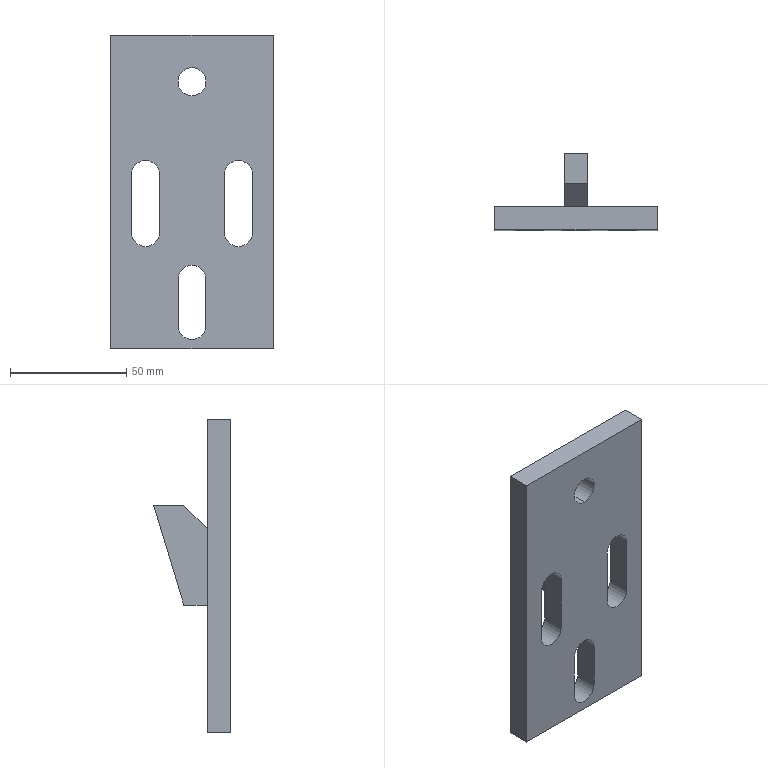Part | SolidWorks | features MirrorStock 1 | 2 solids | 30 faces | box 70 x 33 x 135 mm | volume 88171 mm3 | plane 19 | cylinder 11 | commonest cylinder face diameters 12 x11
STEP:
#1=CARTESIAN_POINT('',(20.,10.,13.5));
#2=VERTEX_POINT('',#1);
#3=CARTESIAN_POINT('',(14.,10.,7.5));
#4=VERTEX_POINT('',#3);
#5=CARTESIAN_POINT('',(20.,10.,7.5));
#6=DIRECTION('',(0.,-1.,0.));
#7=DIRECTION('',(0.,0.,1.));
#8=AXIS2_PLACEMENT_3D('',#5,#6,#7);
#9=CIRCLE('',#8,6.);
#10=EDGE_CURVE('',#2,#4,#9,.T.);
#11=ORIENTED_EDGE('',*,*,#10,.F.);
#12=CARTESIAN_POINT('',(20.,0.,13.5));
#13=VERTEX_POINT('',#12);
#14=CARTESIAN_POINT('',(20.,10.,13.5));
#15=DIRECTION('',(0.,-1.,0.));
#16=VECTOR('',#15,1000.);
#17=LINE('',#14,#16);
#18=EDGE_CURVE('',#2,#13,#17,.T.);
#19=ORIENTED_EDGE('',*,*,#18,.T.);
#20=CARTESIAN_POINT('',(14.,0.,7.5));
#21=VERTEX_POINT('',#20);
#22=CARTESIAN_POINT('',(20.,0.,7.5));
#23=DIRECTION('',(0.,-1.,0.));
#24=DIRECTION('',(0.,0.,1.));
#25=AXIS2_PLACEMENT_3D('',#22,#23,#24);
#26=CIRCLE('',#25,6.);
#27=EDGE_CURVE('',#13,#21,#26,.T.);
#28=ORIENTED_EDGE('',*,*,#27,.T.);
#29=CARTESIAN_POINT('',(14.,10.,7.5));
#30=DIRECTION('',(0.,-1.,0.));
#31=VECTOR('',#30,1000.);
#32=LINE('',#29,#31);
#33=EDGE_CURVE('',#4,#21,#32,.T.);
#34=ORIENTED_EDGE('',*,*,#33,.F.);
#35=EDGE_LOOP('',(#11,#19,#28,#34));
#36=FACE_OUTER_BOUND('',#35,.T.);
#37=CARTESIAN_POINT('',(20.,10.,7.5));
#38=DIRECTION('',(0.,-1.,0.));
#39=DIRECTION('',(0.,0.,1.));
#40=AXIS2_PLACEMENT_3D('',#37,#38,#39);
#41=CYLINDRICAL_SURFACE('',#40,6.);
#42=ADVANCED_FACE('',(#36),#41,.F.);
#43=CARTESIAN_POINT('',(-20.,10.,13.5));
#44=VERTEX_POINT('',#43);
#45=CARTESIAN_POINT('',(-26.,10.,7.5));
#46=VERTEX_POINT('',#45);
#47=CARTESIAN_POINT('',(-20.,10.,7.5));
#48=DIRECTION('',(0.,-1.,0.));
#49=DIRECTION('',(0.,0.,-1.));
#50=AXIS2_PLACEMENT_3D('',#47,#48,#49);
#51=CIRCLE('',#50,6.);
#52=EDGE_CURVE('',#44,#46,#51,.T.);
#53=ORIENTED_EDGE('',*,*,#52,.F.);
#54=CARTESIAN_POINT('',(-20.,0.,13.5));
#55=VERTEX_POINT('',#54);
#56=CARTESIAN_POINT('',(-20.,10.,13.5));
#57=DIRECTION('',(0.,-1.,0.));
#58=VECTOR('',#57,1000.);
#59=LINE('',#56,#58);
#60=EDGE_CURVE('',#44,#55,#59,.T.);
#61=ORIENTED_EDGE('',*,*,#60,.T.);
#62=CARTESIAN_POINT('',(-26.,0.,7.5));
#63=VERTEX_POINT('',#62);
#64=CARTESIAN_POINT('',(-20.,0.,7.5));
#65=DIRECTION('',(0.,-1.,0.));
#66=DIRECTION('',(0.,0.,-1.));
#67=AXIS2_PLACEMENT_3D('',#64,#65,#66);
#68=CIRCLE('',#67,6.);
#69=EDGE_CURVE('',#55,#63,#68,.T.);
#70=ORIENTED_EDGE('',*,*,#69,.T.);
#71=CARTESIAN_POINT('',(-26.,10.,7.5));
#72=DIRECTION('',(0.,-1.,0.));
#73=VECTOR('',#72,1000.);
#74=LINE('',#71,#73);
#75=EDGE_CURVE('',#46,#63,#74,.T.);
#76=ORIENTED_EDGE('',*,*,#75,.F.);
#77=EDGE_LOOP('',(#53,#61,#70,#76));
#78=FACE_OUTER_BOUND('',#77,.T.);
#79=CARTESIAN_POINT('',(-20.,10.,7.5));
#80=DIRECTION('',(0.,-1.,0.));
#81=DIRECTION('',(0.,0.,1.));
#82=AXIS2_PLACEMENT_3D('',#79,#80,#81);
#83=CYLINDRICAL_SURFACE('',#82,6.);
#84=ADVANCED_FACE('',(#78),#83,.F.);
#85=CARTESIAN_POINT('',(0.,10.,-31.5));
#86=VERTEX_POINT('',#85);
#87=CARTESIAN_POINT('',(-6.,10.,-37.5));
#88=VERTEX_POINT('',#87);
#89=CARTESIAN_POINT('',(0.,10.,-37.5));
#90=DIRECTION('',(0.,-1.,0.));
#91=DIRECTION('',(0.,0.,-1.));
#92=AXIS2_PLACEMENT_3D('',#89,#90,#91);
#93=CIRCLE('',#92,6.);
#94=EDGE_CURVE('',#86,#88,#93,.T.);
#95=ORIENTED_EDGE('',*,*,#94,.F.);
#96=CARTESIAN_POINT('',(0.,0.,-31.5));
#97=VERTEX_POINT('',#96);
#98=CARTESIAN_POINT('',(0.,10.,-31.5));
#99=DIRECTION('',(0.,-1.,0.));
#100=VECTOR('',#99,1000.);
#101=LINE('',#98,#100);
#102=EDGE_CURVE('',#86,#97,#101,.T.);
#103=ORIENTED_EDGE('',*,*,#102,.T.);
#104=CARTESIAN_POINT('',(-6.,0.,-37.5));
#105=VERTEX_POINT('',#104);
#106=CARTESIAN_POINT('',(0.,0.,-37.5));
#107=DIRECTION('',(0.,-1.,0.));
#108=DIRECTION('',(0.,0.,-1.));
#109=AXIS2_PLACEMENT_3D('',#106,#107,#108);
#110=CIRCLE('',#109,6.);
#111=EDGE_CURVE('',#97,#105,#110,.T.);
#112=ORIENTED_EDGE('',*,*,#111,.T.);
#113=CARTESIAN_POINT('',(-6.,10.,-37.5));
#114=DIRECTION('',(0.,-1.,0.));
#115=VECTOR('',#114,1000.);
#116=LINE('',#113,#115);
#117=EDGE_CURVE('',#88,#105,#116,.T.);
#118=ORIENTED_EDGE('',*,*,#117,.F.);
#119=EDGE_LOOP('',(#95,#103,#112,#118));
#120=FACE_OUTER_BOUND('',#119,.T.);
#121=CARTESIAN_POINT('',(0.,10.,-37.5));
#122=DIRECTION('',(0.,-1.,0.));
#123=DIRECTION('',(0.,0.,1.));
#124=AXIS2_PLACEMENT_3D('',#121,#122,#123);
#125=CYLINDRICAL_SURFACE('',#124,6.);
#126=ADVANCED_FACE('',(#120),#125,.F.);
#127=CARTESIAN_POINT('',(0.,10.,41.5));
#128=VERTEX_POINT('',#127);
#129=CARTESIAN_POINT('',(0.,10.,53.5));
#130=VERTEX_POINT('',#129);
#131=CARTESIAN_POINT('',(0.,10.,47.5));
#132=DIRECTION('',(0.,-1.,0.));
#133=DIRECTION('',(0.,0.,-1.));
#134=AXIS2_PLACEMENT_3D('',#131,#132,#133);
#135=CIRCLE('',#134,6.);
#136=EDGE_CURVE('',#128,#130,#135,.T.);
#137=ORIENTED_EDGE('',*,*,#136,.F.);
#138=CARTESIAN_POINT('',(0.,0.,41.5));
#139=VERTEX_POINT('',#138);
#140=CARTESIAN_POINT('',(0.,10.,41.5));
#141=DIRECTION('',(0.,-1.,0.));
#142=VECTOR('',#141,1000.);
#143=LINE('',#140,#142);
#144=EDGE_CURVE('',#128,#139,#143,.T.);
#145=ORIENTED_EDGE('',*,*,#144,.T.);
#146=CARTESIAN_POINT('',(0.,0.,53.5));
#147=VERTEX_POINT('',#146);
#148=CARTESIAN_POINT('',(0.,0.,47.5));
#149=DIRECTION('',(0.,-1.,0.));
#150=DIRECTION('',(0.,0.,-1.));
#151=AXIS2_PLACEMENT_3D('',#148,#149,#150);
#152=CIRCLE('',#151,6.);
#153=EDGE_CURVE('',#139,#147,#152,.T.);
#154=ORIENTED_EDGE('',*,*,#153,.T.);
#155=CARTESIAN_POINT('',(0.,10.,53.5));
#156=DIRECTION('',(0.,-1.,0.));
#157=VECTOR('',#156,1000.);
#158=LINE('',#155,#157);
#159=EDGE_CURVE('',#130,#147,#158,.T.);
#160=ORIENTED_EDGE('',*,*,#159,.F.);
#161=EDGE_LOOP('',(#137,#145,#154,#160));
#162=FACE_OUTER_BOUND('',#161,.T.);
#163=CARTESIAN_POINT('',(0.,10.,47.5));
#164=DIRECTION('',(0.,-1.,0.));
#165=DIRECTION('',(0.,0.,1.));
#166=AXIS2_PLACEMENT_3D('',#163,#164,#165);
#167=CYLINDRICAL_SURFACE('',#166,6.);
#168=ADVANCED_FACE('',(#162),#167,.F.);
#169=CARTESIAN_POINT('',(-14.,10.,7.5));
#170=VERTEX_POINT('',#169);
#171=CARTESIAN_POINT('',(-20.,10.,7.5));
#172=DIRECTION('',(0.,-1.,0.));
#173=DIRECTION('',(0.,0.,-1.));
#174=AXIS2_PLACEMENT_3D('',#171,#172,#173);
#175=CIRCLE('',#174,6.);
#176=EDGE_CURVE('',#170,#44,#175,.T.);
#177=ORIENTED_EDGE('',*,*,#176,.T.);
#178=ORIENTED_EDGE('',*,*,#52,.T.);
#179=CARTESIAN_POINT('',(-26.,10.,-17.5));
#180=VERTEX_POINT('',#179);
#181=CARTESIAN_POINT('',(-26.,10.,7.5));
#182=DIRECTION('',(0.,0.,-1.));
#183=VECTOR('',#182,1000.);
#184=LINE('',#181,#183);
#185=EDGE_CURVE('',#46,#180,#184,.T.);
#186=ORIENTED_EDGE('',*,*,#185,.T.);
#187=CARTESIAN_POINT('',(-14.,10.,-17.5));
#188=VERTEX_POINT('',#187);
#189=CARTESIAN_POINT('',(-20.,10.,-17.5));
#190=DIRECTION('',(0.,-1.,0.));
#191=DIRECTION('',(0.,0.,-1.));
#192=AXIS2_PLACEMENT_3D('',#189,#190,#191);
#193=CIRCLE('',#192,6.);
#194=EDGE_CURVE('',#180,#188,#193,.T.);
#195=ORIENTED_EDGE('',*,*,#194,.T.);
#196=CARTESIAN_POINT('',(-14.,10.,7.5));
#197=DIRECTION('',(0.,0.,1.));
#198=VECTOR('',#197,1000.);
#199=LINE('',#196,#198);
#200=EDGE_CURVE('',#188,#170,#199,.T.);
#201=ORIENTED_EDGE('',*,*,#200,.T.);
#202=EDGE_LOOP('',(#177,#178,#186,#195,#201));
#203=FACE_BOUND('',#202,.T.);
#204=CARTESIAN_POINT('',(0.,10.,47.5));
#205=DIRECTION('',(0.,-1.,0.));
#206=DIRECTION('',(0.,0.,-1.));
#207=AXIS2_PLACEMENT_3D('',#204,#205,#206);
#208=CIRCLE('',#207,6.);
#209=EDGE_CURVE('',#130,#128,#208,.T.);
#210=ORIENTED_EDGE('',*,*,#209,.T.);
#211=ORIENTED_EDGE('',*,*,#136,.T.);
#212=EDGE_LOOP('',(#210,#211));
#213=FACE_BOUND('',#212,.T.);
#214=CARTESIAN_POINT('',(35.,10.,-67.5));
#215=VERTEX_POINT('',#214);
#216=CARTESIAN_POINT('',(35.,10.,67.5));
#217=VERTEX_POINT('',#216);
#218=CARTESIAN_POINT('',(35.,10.,-67.5));
#219=DIRECTION('',(0.,0.,1.));
#220=VECTOR('',#219,1000.);
#221=LINE('',#218,#220);
#222=EDGE_CURVE('',#215,#217,#221,.T.);
#223=ORIENTED_EDGE('',*,*,#222,.F.);
#224=CARTESIAN_POINT('',(-35.,10.,-67.5));
#225=VERTEX_POINT('',#224);
#226=CARTESIAN_POINT('',(-35.,10.,-67.5));
#227=DIRECTION('',(1.,0.,0.));
#228=VECTOR('',#227,1000.);
#229=LINE('',#226,#228);
#230=EDGE_CURVE('',#225,#215,#229,.T.);
#231=ORIENTED_EDGE('',*,*,#230,.F.);
#232=CARTESIAN_POINT('',(-35.,10.,67.5));
#233=VERTEX_POINT('',#232);
#234=CARTESIAN_POINT('',(-35.,10.,-67.5));
#235=DIRECTION('',(0.,0.,-1.));
#236=VECTOR('',#235,1000.);
#237=LINE('',#234,#236);
#238=EDGE_CURVE('',#233,#225,#237,.T.);
#239=ORIENTED_EDGE('',*,*,#238,.F.);
#240=CARTESIAN_POINT('',(-35.,10.,67.5));
#241=DIRECTION('',(-1.,0.,0.));
#242=VECTOR('',#241,1000.);
#243=LINE('',#240,#242);
#244=EDGE_CURVE('',#217,#233,#243,.T.);
#245=ORIENTED_EDGE('',*,*,#244,.F.);
#246=EDGE_LOOP('',(#223,#231,#239,#245));
#247=FACE_OUTER_BOUND('',#246,.T.);
#248=CARTESIAN_POINT('',(6.,10.,-37.5));
#249=VERTEX_POINT('',#248);
#250=CARTESIAN_POINT('',(0.,10.,-37.5));
#251=DIRECTION('',(0.,-1.,0.));
#252=DIRECTION('',(0.,0.,-1.));
#253=AXIS2_PLACEMENT_3D('',#250,#251,#252);
#254=CIRCLE('',#253,6.);
#255=EDGE_CURVE('',#249,#86,#254,.T.);
#256=ORIENTED_EDGE('',*,*,#255,.T.);
#257=ORIENTED_EDGE('',*,*,#94,.T.);
#258=CARTESIAN_POINT('',(-6.,10.,-57.5));
#259=VERTEX_POINT('',#258);
#260=CARTESIAN_POINT('',(-6.,10.,-37.5));
#261=DIRECTION('',(0.,0.,-1.));
#262=VECTOR('',#261,1000.);
#263=LINE('',#260,#262);
#264=EDGE_CURVE('',#88,#259,#263,.T.);
#265=ORIENTED_EDGE('',*,*,#264,.T.);
#266=CARTESIAN_POINT('',(6.,10.,-57.5));
#267=VERTEX_POINT('',#266);
#268=CARTESIAN_POINT('',(0.,10.,-57.5));
#269=DIRECTION('',(0.,-1.,0.));
#270=DIRECTION('',(0.,0.,-1.));
#271=AXIS2_PLACEMENT_3D('',#268,#269,#270);
#272=CIRCLE('',#271,6.);
#273=EDGE_CURVE('',#259,#267,#272,.T.);
#274=ORIENTED_EDGE('',*,*,#273,.T.);
#275=CARTESIAN_POINT('',(6.,10.,-37.5));
#276=DIRECTION('',(0.,0.,1.));
#277=VECTOR('',#276,1000.);
#278=LINE('',#275,#277);
#279=EDGE_CURVE('',#267,#249,#278,.T.);
#280=ORIENTED_EDGE('',*,*,#279,.T.);
#281=EDGE_LOOP('',(#256,#257,#265,#274,#280));
#282=FACE_BOUND('',#281,.T.);
#283=CARTESIAN_POINT('',(26.,10.,7.5));
#284=VERTEX_POINT('',#283);
#285=CARTESIAN_POINT('',(20.,10.,7.5));
#286=DIRECTION('',(0.,-1.,0.));
#287=DIRECTION('',(0.,0.,1.));
#288=AXIS2_PLACEMENT_3D('',#285,#286,#287);
#289=CIRCLE('',#288,6.);
#290=EDGE_CURVE('',#284,#2,#289,.T.);
#291=ORIENTED_EDGE('',*,*,#290,.T.);
#292=ORIENTED_EDGE('',*,*,#10,.T.);
#293=CARTESIAN_POINT('',(14.,10.,-17.5));
#294=VERTEX_POINT('',#293);
#295=CARTESIAN_POINT('',(14.,10.,7.5));
#296=DIRECTION('',(0.,0.,-1.));
#297=VECTOR('',#296,1000.);
#298=LINE('',#295,#297);
#299=EDGE_CURVE('',#4,#294,#298,.T.);
#300=ORIENTED_EDGE('',*,*,#299,.T.);
#301=CARTESIAN_POINT('',(26.,10.,-17.5));
#302=VERTEX_POINT('',#301);
#303=CARTESIAN_POINT('',(20.,10.,-17.5));
#304=DIRECTION('',(0.,-1.,0.));
#305=DIRECTION('',(0.,0.,1.));
#306=AXIS2_PLACEMENT_3D('',#303,#304,#305);
#307=CIRCLE('',#306,6.);
#308=EDGE_CURVE('',#294,#302,#307,.T.);
#309=ORIENTED_EDGE('',*,*,#308,.T.);
#310=CARTESIAN_POINT('',(26.,10.,7.5));
#311=DIRECTION('',(0.,0.,1.));
#312=VECTOR('',#311,1000.);
#313=LINE('',#310,#312);
#314=EDGE_CURVE('',#302,#284,#313,.T.);
#315=ORIENTED_EDGE('',*,*,#314,.T.);
#316=EDGE_LOOP('',(#291,#292,#300,#309,#315));
#317=FACE_BOUND('',#316,.T.);
#318=CARTESIAN_POINT('',(0.,10.,0.));
#319=DIRECTION('',(0.,-1.,0.));
#320=DIRECTION('',(0.,0.,1.));
#321=AXIS2_PLACEMENT_3D('',#318,#319,#320);
#322=PLANE('',#321);
#323=ADVANCED_FACE('',(#203,#213,#247,#282,#317),#322,.F.);
#324=CARTESIAN_POINT('',(35.,0.,-67.5));
#325=VERTEX_POINT('',#324);
#326=CARTESIAN_POINT('',(35.,0.,67.5));
#327=VERTEX_POINT('',#326);
#328=CARTESIAN_POINT('',(35.,0.,-67.5));
#329=DIRECTION('',(0.,0.,1.));
#330=VECTOR('',#329,1000.);
#331=LINE('',#328,#330);
#332=EDGE_CURVE('',#325,#327,#331,.T.);
#333=ORIENTED_EDGE('',*,*,#332,.T.);
#334=CARTESIAN_POINT('',(-35.,0.,67.5));
#335=VERTEX_POINT('',#334);
#336=CARTESIAN_POINT('',(-35.,0.,67.5));
#337=DIRECTION('',(-1.,0.,0.));
#338=VECTOR('',#337,1000.);
#339=LINE('',#336,#338);
#340=EDGE_CURVE('',#327,#335,#339,.T.);
#341=ORIENTED_EDGE('',*,*,#340,.T.);
#342=CARTESIAN_POINT('',(-35.,0.,-67.5));
#343=VERTEX_POINT('',#342);
#344=CARTESIAN_POINT('',(-35.,0.,-67.5));
#345=DIRECTION('',(0.,0.,-1.));
#346=VECTOR('',#345,1000.);
#347=LINE('',#344,#346);
#348=EDGE_CURVE('',#335,#343,#347,.T.);
#349=ORIENTED_EDGE('',*,*,#348,.T.);
#350=CARTESIAN_POINT('',(-35.,0.,-67.5));
#351=DIRECTION('',(1.,0.,0.));
#352=VECTOR('',#351,1000.);
#353=LINE('',#350,#352);
#354=EDGE_CURVE('',#343,#325,#353,.T.);
#355=ORIENTED_EDGE('',*,*,#354,.T.);
#356=EDGE_LOOP('',(#333,#341,#349,#355));
#357=FACE_OUTER_BOUND('',#356,.T.);
#358=CARTESIAN_POINT('',(0.,0.,47.5));
#359=DIRECTION('',(0.,-1.,0.));
#360=DIRECTION('',(0.,0.,-1.));
#361=AXIS2_PLACEMENT_3D('',#358,#359,#360);
#362=CIRCLE('',#361,6.);
#363=EDGE_CURVE('',#147,#139,#362,.T.);
#364=ORIENTED_EDGE('',*,*,#363,.F.);
#365=ORIENTED_EDGE('',*,*,#153,.F.);
#366=EDGE_LOOP('',(#364,#365));
#367=FACE_BOUND('',#366,.T.);
#368=CARTESIAN_POINT('',(6.,0.,-57.5));
#369=VERTEX_POINT('',#368);
#370=CARTESIAN_POINT('',(6.,0.,-37.5));
#371=VERTEX_POINT('',#370);
#372=CARTESIAN_POINT('',(6.,0.,-37.5));
#373=DIRECTION('',(0.,0.,1.));
#374=VECTOR('',#373,1000.);
#375=LINE('',#372,#374);
#376=EDGE_CURVE('',#369,#371,#375,.T.);
#377=ORIENTED_EDGE('',*,*,#376,.F.);
#378=CARTESIAN_POINT('',(-6.,0.,-57.5));
#379=VERTEX_POINT('',#378);
#380=CARTESIAN_POINT('',(0.,0.,-57.5));
#381=DIRECTION('',(0.,-1.,0.));
#382=DIRECTION('',(0.,0.,-1.));
#383=AXIS2_PLACEMENT_3D('',#380,#381,#382);
#384=CIRCLE('',#383,6.);
#385=EDGE_CURVE('',#379,#369,#384,.T.);
#386=ORIENTED_EDGE('',*,*,#385,.F.);
#387=CARTESIAN_POINT('',(-6.,0.,-37.5));
#388=DIRECTION('',(0.,0.,-1.));
#389=VECTOR('',#388,1000.);
#390=LINE('',#387,#389);
#391=EDGE_CURVE('',#105,#379,#390,.T.);
#392=ORIENTED_EDGE('',*,*,#391,.F.);
#393=ORIENTED_EDGE('',*,*,#111,.F.);
#394=CARTESIAN_POINT('',(0.,0.,-37.5));
#395=DIRECTION('',(0.,-1.,0.));
#396=DIRECTION('',(0.,0.,-1.));
#397=AXIS2_PLACEMENT_3D('',#394,#395,#396);
#398=CIRCLE('',#397,6.);
#399=EDGE_CURVE('',#371,#97,#398,.T.);
#400=ORIENTED_EDGE('',*,*,#399,.F.);
#401=EDGE_LOOP('',(#377,#386,#392,#393,#400));
#402=FACE_BOUND('',#401,.T.);
#403=CARTESIAN_POINT('',(-14.,0.,-17.5));
#404=VERTEX_POINT('',#403);
#405=CARTESIAN_POINT('',(-14.,0.,7.5));
#406=VERTEX_POINT('',#405);
#407=CARTESIAN_POINT('',(-14.,0.,7.5));
#408=DIRECTION('',(0.,0.,1.));
#409=VECTOR('',#408,1000.);
#410=LINE('',#407,#409);
#411=EDGE_CURVE('',#404,#406,#410,.T.);
#412=ORIENTED_EDGE('',*,*,#411,.F.);
#413=CARTESIAN_POINT('',(-26.,0.,-17.5));
#414=VERTEX_POINT('',#413);
#415=CARTESIAN_POINT('',(-20.,0.,-17.5));
#416=DIRECTION('',(0.,-1.,0.));
#417=DIRECTION('',(0.,0.,-1.));
#418=AXIS2_PLACEMENT_3D('',#415,#416,#417);
#419=CIRCLE('',#418,6.);
#420=EDGE_CURVE('',#414,#404,#419,.T.);
#421=ORIENTED_EDGE('',*,*,#420,.F.);
#422=CARTESIAN_POINT('',(-26.,0.,7.5));
#423=DIRECTION('',(0.,0.,-1.));
#424=VECTOR('',#423,1000.);
#425=LINE('',#422,#424);
#426=EDGE_CURVE('',#63,#414,#425,.T.);
#427=ORIENTED_EDGE('',*,*,#426,.F.);
#428=ORIENTED_EDGE('',*,*,#69,.F.);
#429=CARTESIAN_POINT('',(-20.,0.,7.5));
#430=DIRECTION('',(0.,-1.,0.));
#431=DIRECTION('',(0.,0.,-1.));
#432=AXIS2_PLACEMENT_3D('',#429,#430,#431);
#433=CIRCLE('',#432,6.);
#434=EDGE_CURVE('',#406,#55,#433,.T.);
#435=ORIENTED_EDGE('',*,*,#434,.F.);
#436=EDGE_LOOP('',(#412,#421,#427,#428,#435));
#437=FACE_BOUND('',#436,.T.);
#438=CARTESIAN_POINT('',(26.,0.,-17.5));
#439=VERTEX_POINT('',#438);
#440=CARTESIAN_POINT('',(26.,0.,7.5));
#441=VERTEX_POINT('',#440);
#442=CARTESIAN_POINT('',(26.,0.,7.5));
#443=DIRECTION('',(0.,0.,1.));
#444=VECTOR('',#443,1000.);
#445=LINE('',#442,#444);
#446=EDGE_CURVE('',#439,#441,#445,.T.);
#447=ORIENTED_EDGE('',*,*,#446,.F.);
#448=CARTESIAN_POINT('',(14.,0.,-17.5));
#449=VERTEX_POINT('',#448);
#450=CARTESIAN_POINT('',(20.,0.,-17.5));
#451=DIRECTION('',(0.,-1.,0.));
#452=DIRECTION('',(0.,0.,1.));
#453=AXIS2_PLACEMENT_3D('',#450,#451,#452);
#454=CIRCLE('',#453,6.);
#455=EDGE_CURVE('',#449,#439,#454,.T.);
#456=ORIENTED_EDGE('',*,*,#455,.F.);
#457=CARTESIAN_POINT('',(14.,0.,7.5));
#458=DIRECTION('',(0.,0.,-1.));
#459=VECTOR('',#458,1000.);
#460=LINE('',#457,#459);
#461=EDGE_CURVE('',#21,#449,#460,.T.);
#462=ORIENTED_EDGE('',*,*,#461,.F.);
#463=ORIENTED_EDGE('',*,*,#27,.F.);
#464=CARTESIAN_POINT('',(20.,0.,7.5));
#465=DIRECTION('',(0.,-1.,0.));
#466=DIRECTION('',(0.,0.,1.));
#467=AXIS2_PLACEMENT_3D('',#464,#465,#466);
#468=CIRCLE('',#467,6.);
#469=EDGE_CURVE('',#441,#13,#468,.T.);
#470=ORIENTED_EDGE('',*,*,#469,.F.);
#471=EDGE_LOOP('',(#447,#456,#462,#463,#470));
#472=FACE_BOUND('',#471,.T.);
#473=CARTESIAN_POINT('',(0.,0.,0.));
#474=DIRECTION('',(0.,-1.,0.));
#475=DIRECTION('',(0.,0.,1.));
#476=AXIS2_PLACEMENT_3D('',#473,#474,#475);
#477=PLANE('',#476);
#478=ADVANCED_FACE('',(#357,#367,#402,#437,#472),#477,.T.);
#479=ORIENTED_EDGE('',*,*,#332,.F.);
#480=CARTESIAN_POINT('',(35.,10.,-67.5));
#481=DIRECTION('',(0.,-1.,0.));
#482=VECTOR('',#481,1000.);
#483=LINE('',#480,#482);
#484=EDGE_CURVE('',#215,#325,#483,.T.);
#485=ORIENTED_EDGE('',*,*,#484,.F.);
#486=ORIENTED_EDGE('',*,*,#222,.T.);
#487=CARTESIAN_POINT('',(35.,10.,67.5));
#488=DIRECTION('',(0.,-1.,0.));
#489=VECTOR('',#488,1000.);
#490=LINE('',#487,#489);
#491=EDGE_CURVE('',#217,#327,#490,.T.);
#492=ORIENTED_EDGE('',*,*,#491,.T.);
#493=EDGE_LOOP('',(#479,#485,#486,#492));
#494=FACE_OUTER_BOUND('',#493,.T.);
#495=CARTESIAN_POINT('',(35.,10.,-67.5));
#496=DIRECTION('',(-1.,0.,0.));
#497=DIRECTION('',(0.,0.,-1.));
#498=AXIS2_PLACEMENT_3D('',#495,#496,#497);
#499=PLANE('',#498);
#500=ADVANCED_FACE('',(#494),#499,.F.);
#501=ORIENTED_EDGE('',*,*,#340,.F.);
#502=ORIENTED_EDGE('',*,*,#491,.F.);
#503=ORIENTED_EDGE('',*,*,#244,.T.);
#504=CARTESIAN_POINT('',(-35.,10.,67.5));
#505=DIRECTION('',(0.,-1.,0.));
#506=VECTOR('',#505,1000.);
#507=LINE('',#504,#506);
#508=EDGE_CURVE('',#233,#335,#507,.T.);
#509=ORIENTED_EDGE('',*,*,#508,.T.);
#510=EDGE_LOOP('',(#501,#502,#503,#509));
#511=FACE_OUTER_BOUND('',#510,.T.);
#512=CARTESIAN_POINT('',(-35.,10.,67.5));
#513=DIRECTION('',(0.,0.,-1.));
#514=DIRECTION('',(1.,0.,0.));
#515=AXIS2_PLACEMENT_3D('',#512,#513,#514);
#516=PLANE('',#515);
#517=ADVANCED_FACE('',(#511),#516,.F.);
#518=ORIENTED_EDGE('',*,*,#348,.F.);
#519=ORIENTED_EDGE('',*,*,#508,.F.);
#520=ORIENTED_EDGE('',*,*,#238,.T.);
#521=CARTESIAN_POINT('',(-35.,10.,-67.5));
#522=DIRECTION('',(0.,-1.,0.));
#523=VECTOR('',#522,1000.);
#524=LINE('',#521,#523);
#525=EDGE_CURVE('',#225,#343,#524,.T.);
#526=ORIENTED_EDGE('',*,*,#525,.T.);
#527=EDGE_LOOP('',(#518,#519,#520,#526));
#528=FACE_OUTER_BOUND('',#527,.T.);
#529=CARTESIAN_POINT('',(-35.,10.,-67.5));
#530=DIRECTION('',(1.,0.,0.));
#531=DIRECTION('',(0.,0.,1.));
#532=AXIS2_PLACEMENT_3D('',#529,#530,#531);
#533=PLANE('',#532);
#534=ADVANCED_FACE('',(#528),#533,.F.);
#535=ORIENTED_EDGE('',*,*,#354,.F.);
#536=ORIENTED_EDGE('',*,*,#525,.F.);
#537=ORIENTED_EDGE('',*,*,#230,.T.);
#538=ORIENTED_EDGE('',*,*,#484,.T.);
#539=EDGE_LOOP('',(#535,#536,#537,#538));
#540=FACE_OUTER_BOUND('',#539,.T.);
#541=CARTESIAN_POINT('',(-35.,10.,-67.5));
#542=DIRECTION('',(0.,0.,1.));
#543=DIRECTION('',(-1.,0.,0.));
#544=AXIS2_PLACEMENT_3D('',#541,#542,#543);
#545=PLANE('',#544);
#546=ADVANCED_FACE('',(#540),#545,.F.);
#547=ORIENTED_EDGE('',*,*,#144,.F.);
#548=ORIENTED_EDGE('',*,*,#209,.F.);
#549=ORIENTED_EDGE('',*,*,#159,.T.);
#550=ORIENTED_EDGE('',*,*,#363,.T.);
#551=EDGE_LOOP('',(#547,#548,#549,#550));
#552=FACE_OUTER_BOUND('',#551,.T.);
#553=CARTESIAN_POINT('',(0.,10.,47.5));
#554=DIRECTION('',(0.,-1.,0.));
#555=DIRECTION('',(0.,0.,1.));
#556=AXIS2_PLACEMENT_3D('',#553,#554,#555);
#557=CYLINDRICAL_SURFACE('',#556,6.);
#558=ADVANCED_FACE('',(#552),#557,.F.);
#559=ORIENTED_EDGE('',*,*,#102,.F.);
#560=ORIENTED_EDGE('',*,*,#255,.F.);
#561=CARTESIAN_POINT('',(6.,10.,-37.5));
#562=DIRECTION('',(0.,-1.,0.));
#563=VECTOR('',#562,1000.);
#564=LINE('',#561,#563);
#565=EDGE_CURVE('',#249,#371,#564,.T.);
#566=ORIENTED_EDGE('',*,*,#565,.T.);
#567=ORIENTED_EDGE('',*,*,#399,.T.);
#568=EDGE_LOOP('',(#559,#560,#566,#567));
#569=FACE_OUTER_BOUND('',#568,.T.);
#570=CARTESIAN_POINT('',(0.,10.,-37.5));
#571=DIRECTION('',(0.,-1.,0.));
#572=DIRECTION('',(0.,0.,1.));
#573=AXIS2_PLACEMENT_3D('',#570,#571,#572);
#574=CYLINDRICAL_SURFACE('',#573,6.);
#575=ADVANCED_FACE('',(#569),#574,.F.);
#576=ORIENTED_EDGE('',*,*,#391,.T.);
#577=CARTESIAN_POINT('',(-6.,10.,-57.5));
#578=DIRECTION('',(0.,-1.,0.));
#579=VECTOR('',#578,1000.);
#580=LINE('',#577,#579);
#581=EDGE_CURVE('',#259,#379,#580,.T.);
#582=ORIENTED_EDGE('',*,*,#581,.F.);
#583=ORIENTED_EDGE('',*,*,#264,.F.);
#584=ORIENTED_EDGE('',*,*,#117,.T.);
#585=EDGE_LOOP('',(#576,#582,#583,#584));
#586=FACE_OUTER_BOUND('',#585,.T.);
#587=CARTESIAN_POINT('',(-6.,10.,-37.5));
#588=DIRECTION('',(1.,0.,0.));
#589=DIRECTION('',(0.,0.,1.));
#590=AXIS2_PLACEMENT_3D('',#587,#588,#589);
#591=PLANE('',#590);
#592=ADVANCED_FACE('',(#586),#591,.T.);
#593=ORIENTED_EDGE('',*,*,#385,.T.);
#594=CARTESIAN_POINT('',(6.,10.,-57.5));
#595=DIRECTION('',(0.,-1.,0.));
#596=VECTOR('',#595,1000.);
#597=LINE('',#594,#596);
#598=EDGE_CURVE('',#267,#369,#597,.T.);
#599=ORIENTED_EDGE('',*,*,#598,.F.);
#600=ORIENTED_EDGE('',*,*,#273,.F.);
#601=ORIENTED_EDGE('',*,*,#581,.T.);
#602=EDGE_LOOP('',(#593,#599,#600,#601));
#603=FACE_OUTER_BOUND('',#602,.T.);
#604=CARTESIAN_POINT('',(0.,10.,-57.5));
#605=DIRECTION('',(0.,-1.,0.));
#606=DIRECTION('',(0.,0.,1.));
#607=AXIS2_PLACEMENT_3D('',#604,#605,#606);
#608=CYLINDRICAL_SURFACE('',#607,6.);
#609=ADVANCED_FACE('',(#603),#608,.F.);
#610=ORIENTED_EDGE('',*,*,#376,.T.);
#611=ORIENTED_EDGE('',*,*,#565,.F.);
#612=ORIENTED_EDGE('',*,*,#279,.F.);
#613=ORIENTED_EDGE('',*,*,#598,.T.);
#614=EDGE_LOOP('',(#610,#611,#612,#613));
#615=FACE_OUTER_BOUND('',#614,.T.);
#616=CARTESIAN_POINT('',(6.,10.,-37.5));
#617=DIRECTION('',(-1.,0.,0.));
#618=DIRECTION('',(0.,0.,-1.));
#619=AXIS2_PLACEMENT_3D('',#616,#617,#618);
#620=PLANE('',#619);
#621=ADVANCED_FACE('',(#615),#620,.T.);
#622=ORIENTED_EDGE('',*,*,#60,.F.);
#623=ORIENTED_EDGE('',*,*,#176,.F.);
#624=CARTESIAN_POINT('',(-14.,10.,7.5));
#625=DIRECTION('',(0.,-1.,0.));
#626=VECTOR('',#625,1000.);
#627=LINE('',#624,#626);
#628=EDGE_CURVE('',#170,#406,#627,.T.);
#629=ORIENTED_EDGE('',*,*,#628,.T.);
#630=ORIENTED_EDGE('',*,*,#434,.T.);
#631=EDGE_LOOP('',(#622,#623,#629,#630));
#632=FACE_OUTER_BOUND('',#631,.T.);
#633=CARTESIAN_POINT('',(-20.,10.,7.5));
#634=DIRECTION('',(0.,-1.,0.));
#635=DIRECTION('',(0.,0.,1.));
#636=AXIS2_PLACEMENT_3D('',#633,#634,#635);
#637=CYLINDRICAL_SURFACE('',#636,6.);
#638=ADVANCED_FACE('',(#632),#637,.F.);
#639=ORIENTED_EDGE('',*,*,#426,.T.);
#640=CARTESIAN_POINT('',(-26.,10.,-17.5));
#641=DIRECTION('',(0.,-1.,0.));
#642=VECTOR('',#641,1000.);
#643=LINE('',#640,#642);
#644=EDGE_CURVE('',#180,#414,#643,.T.);
#645=ORIENTED_EDGE('',*,*,#644,.F.);
#646=ORIENTED_EDGE('',*,*,#185,.F.);
#647=ORIENTED_EDGE('',*,*,#75,.T.);
#648=EDGE_LOOP('',(#639,#645,#646,#647));
#649=FACE_OUTER_BOUND('',#648,.T.);
#650=CARTESIAN_POINT('',(-26.,10.,7.5));
#651=DIRECTION('',(1.,0.,0.));
#652=DIRECTION('',(0.,0.,1.));
#653=AXIS2_PLACEMENT_3D('',#650,#651,#652);
#654=PLANE('',#653);
#655=ADVANCED_FACE('',(#649),#654,.T.);
#656=ORIENTED_EDGE('',*,*,#420,.T.);
#657=CARTESIAN_POINT('',(-14.,10.,-17.5));
#658=DIRECTION('',(0.,-1.,0.));
#659=VECTOR('',#658,1000.);
#660=LINE('',#657,#659);
#661=EDGE_CURVE('',#188,#404,#660,.T.);
#662=ORIENTED_EDGE('',*,*,#661,.F.);
#663=ORIENTED_EDGE('',*,*,#194,.F.);
#664=ORIENTED_EDGE('',*,*,#644,.T.);
#665=EDGE_LOOP('',(#656,#662,#663,#664));
#666=FACE_OUTER_BOUND('',#665,.T.);
#667=CARTESIAN_POINT('',(-20.,10.,-17.5));
#668=DIRECTION('',(0.,-1.,0.));
#669=DIRECTION('',(0.,0.,1.));
#670=AXIS2_PLACEMENT_3D('',#667,#668,#669);
#671=CYLINDRICAL_SURFACE('',#670,6.);
#672=ADVANCED_FACE('',(#666),#671,.F.);
#673=ORIENTED_EDGE('',*,*,#411,.T.);
#674=ORIENTED_EDGE('',*,*,#628,.F.);
#675=ORIENTED_EDGE('',*,*,#200,.F.);
#676=ORIENTED_EDGE('',*,*,#661,.T.);
#677=EDGE_LOOP('',(#673,#674,#675,#676));
#678=FACE_OUTER_BOUND('',#677,.T.);
#679=CARTESIAN_POINT('',(-14.,10.,7.5));
#680=DIRECTION('',(-1.,0.,0.));
#681=DIRECTION('',(0.,0.,-1.));
#682=AXIS2_PLACEMENT_3D('',#679,#680,#681);
#683=PLANE('',#682);
#684=ADVANCED_FACE('',(#678),#683,.T.);
#685=ORIENTED_EDGE('',*,*,#18,.F.);
#686=ORIENTED_EDGE('',*,*,#290,.F.);
#687=CARTESIAN_POINT('',(26.,10.,7.5));
#688=DIRECTION('',(0.,-1.,0.));
#689=VECTOR('',#688,1000.);
#690=LINE('',#687,#689);
#691=EDGE_CURVE('',#284,#441,#690,.T.);
#692=ORIENTED_EDGE('',*,*,#691,.T.);
#693=ORIENTED_EDGE('',*,*,#469,.T.);
#694=EDGE_LOOP('',(#685,#686,#692,#693));
#695=FACE_OUTER_BOUND('',#694,.T.);
#696=CARTESIAN_POINT('',(20.,10.,7.5));
#697=DIRECTION('',(0.,-1.,0.));
#698=DIRECTION('',(0.,0.,1.));
#699=AXIS2_PLACEMENT_3D('',#696,#697,#698);
#700=CYLINDRICAL_SURFACE('',#699,6.);
#701=ADVANCED_FACE('',(#695),#700,.F.);
#702=ORIENTED_EDGE('',*,*,#461,.T.);
#703=CARTESIAN_POINT('',(14.,10.,-17.5));
#704=DIRECTION('',(0.,-1.,0.));
#705=VECTOR('',#704,1000.);
#706=LINE('',#703,#705);
#707=EDGE_CURVE('',#294,#449,#706,.T.);
#708=ORIENTED_EDGE('',*,*,#707,.F.);
#709=ORIENTED_EDGE('',*,*,#299,.F.);
#710=ORIENTED_EDGE('',*,*,#33,.T.);
#711=EDGE_LOOP('',(#702,#708,#709,#710));
#712=FACE_OUTER_BOUND('',#711,.T.);
#713=CARTESIAN_POINT('',(14.,10.,7.5));
#714=DIRECTION('',(1.,0.,0.));
#715=DIRECTION('',(0.,0.,1.));
#716=AXIS2_PLACEMENT_3D('',#713,#714,#715);
#717=PLANE('',#716);
#718=ADVANCED_FACE('',(#712),#717,.T.);
#719=ORIENTED_EDGE('',*,*,#455,.T.);
#720=CARTESIAN_POINT('',(26.,10.,-17.5));
#721=DIRECTION('',(0.,-1.,0.));
#722=VECTOR('',#721,1000.);
#723=LINE('',#720,#722);
#724=EDGE_CURVE('',#302,#439,#723,.T.);
#725=ORIENTED_EDGE('',*,*,#724,.F.);
#726=ORIENTED_EDGE('',*,*,#308,.F.);
#727=ORIENTED_EDGE('',*,*,#707,.T.);
#728=EDGE_LOOP('',(#719,#725,#726,#727));
#729=FACE_OUTER_BOUND('',#728,.T.);
#730=CARTESIAN_POINT('',(20.,10.,-17.5));
#731=DIRECTION('',(0.,-1.,0.));
#732=DIRECTION('',(0.,0.,1.));
#733=AXIS2_PLACEMENT_3D('',#730,#731,#732);
#734=CYLINDRICAL_SURFACE('',#733,6.);
#735=ADVANCED_FACE('',(#729),#734,.F.);
#736=ORIENTED_EDGE('',*,*,#446,.T.);
#737=ORIENTED_EDGE('',*,*,#691,.F.);
#738=ORIENTED_EDGE('',*,*,#314,.F.);
#739=ORIENTED_EDGE('',*,*,#724,.T.);
#740=EDGE_LOOP('',(#736,#737,#738,#739));
#741=FACE_OUTER_BOUND('',#740,.T.);
#742=CARTESIAN_POINT('',(26.,10.,7.5));
#743=DIRECTION('',(-1.,0.,0.));
#744=DIRECTION('',(0.,0.,-1.));
#745=AXIS2_PLACEMENT_3D('',#742,#743,#744);
#746=PLANE('',#745);
#747=ADVANCED_FACE('',(#741),#746,.T.);
#748=CLOSED_SHELL('',(#42,#84,#126,#168,#323,#478,#500,#517,#534,#546,#558,#575,#592,#609,#621,#638,#655,#672,#684,#701,#718,#735,#747));
#749=MANIFOLD_SOLID_BREP('',#748);
#750=CARTESIAN_POINT('',(-5.,10.,-12.5));
#751=VERTEX_POINT('',#750);
#752=CARTESIAN_POINT('',(-5.,10.,20.5));
#753=VERTEX_POINT('',#752);
#754=CARTESIAN_POINT('',(-5.,10.,20.5));
#755=DIRECTION('',(0.,0.,1.));
#756=VECTOR('',#755,1000.);
#757=LINE('',#754,#756);
#758=EDGE_CURVE('',#751,#753,#757,.T.);
#759=ORIENTED_EDGE('',*,*,#758,.F.);
#760=CARTESIAN_POINT('',(5.,10.,-12.5));
#761=VERTEX_POINT('',#760);
#762=CARTESIAN_POINT('',(5.,10.,-12.5));
#763=DIRECTION('',(-1.,0.,0.));
#764=VECTOR('',#763,1000.);
#765=LINE('',#762,#764);
#766=EDGE_CURVE('',#761,#751,#765,.T.);
#767=ORIENTED_EDGE('',*,*,#766,.F.);
#768=CARTESIAN_POINT('',(5.,10.,20.5));
#769=VERTEX_POINT('',#768);
#770=CARTESIAN_POINT('',(5.,10.,20.5));
#771=DIRECTION('',(0.,0.,1.));
#772=VECTOR('',#771,1000.);
#773=LINE('',#770,#772);
#774=EDGE_CURVE('',#761,#769,#773,.T.);
#775=ORIENTED_EDGE('',*,*,#774,.T.);
#776=CARTESIAN_POINT('',(5.,10.,20.5));
#777=DIRECTION('',(-1.,0.,0.));
#778=VECTOR('',#777,1000.);
#779=LINE('',#776,#778);
#780=EDGE_CURVE('',#769,#753,#779,.T.);
#781=ORIENTED_EDGE('',*,*,#780,.T.);
#782=EDGE_LOOP('',(#759,#767,#775,#781));
#783=FACE_OUTER_BOUND('',#782,.T.);
#784=CARTESIAN_POINT('',(5.,10.,20.5));
#785=DIRECTION('',(0.,1.,0.));
#786=DIRECTION('',(0.,0.,-1.));
#787=AXIS2_PLACEMENT_3D('',#784,#785,#786);
#788=PLANE('',#787);
#789=ADVANCED_FACE('',(#783),#788,.F.);
#790=CARTESIAN_POINT('',(-5.,20.,30.5));
#791=VERTEX_POINT('',#790);
#792=CARTESIAN_POINT('',(-5.,20.,30.5));
#793=DIRECTION('',(0.,0.7071,0.7071));
#794=VECTOR('',#793,1000.);
#795=LINE('',#792,#794);
#796=EDGE_CURVE('',#753,#791,#795,.T.);
#797=ORIENTED_EDGE('',*,*,#796,.F.);
#798=ORIENTED_EDGE('',*,*,#780,.F.);
#799=CARTESIAN_POINT('',(5.,20.,30.5));
#800=VERTEX_POINT('',#799);
#801=CARTESIAN_POINT('',(5.,20.,30.5));
#802=DIRECTION('',(0.,0.7071,0.7071));
#803=VECTOR('',#802,1000.);
#804=LINE('',#801,#803);
#805=EDGE_CURVE('',#769,#800,#804,.T.);
#806=ORIENTED_EDGE('',*,*,#805,.T.);
#807=CARTESIAN_POINT('',(5.,20.,30.5));
#808=DIRECTION('',(-1.,0.,0.));
#809=VECTOR('',#808,1000.);
#810=LINE('',#807,#809);
#811=EDGE_CURVE('',#800,#791,#810,.T.);
#812=ORIENTED_EDGE('',*,*,#811,.T.);
#813=EDGE_LOOP('',(#797,#798,#806,#812));
#814=FACE_OUTER_BOUND('',#813,.T.);
#815=CARTESIAN_POINT('',(5.,20.,30.5));
#816=DIRECTION('',(0.,0.7071,-0.7071));
#817=DIRECTION('',(0.,-0.7071,-0.7071));
#818=AXIS2_PLACEMENT_3D('',#815,#816,#817);
#819=PLANE('',#818);
#820=ADVANCED_FACE('',(#814),#819,.F.);
#821=CARTESIAN_POINT('',(-5.,33.,30.5));
#822=VERTEX_POINT('',#821);
#823=CARTESIAN_POINT('',(-5.,33.,30.5));
#824=DIRECTION('',(0.,1.,0.));
#825=VECTOR('',#824,1000.);
#826=LINE('',#823,#825);
#827=EDGE_CURVE('',#791,#822,#826,.T.);
#828=ORIENTED_EDGE('',*,*,#827,.F.);
#829=ORIENTED_EDGE('',*,*,#811,.F.);
#830=CARTESIAN_POINT('',(5.,33.,30.5));
#831=VERTEX_POINT('',#830);
#832=CARTESIAN_POINT('',(5.,33.,30.5));
#833=DIRECTION('',(0.,1.,0.));
#834=VECTOR('',#833,1000.);
#835=LINE('',#832,#834);
#836=EDGE_CURVE('',#800,#831,#835,.T.);
#837=ORIENTED_EDGE('',*,*,#836,.T.);
#838=CARTESIAN_POINT('',(5.,33.,30.5));
#839=DIRECTION('',(-1.,0.,0.));
#840=VECTOR('',#839,1000.);
#841=LINE('',#838,#840);
#842=EDGE_CURVE('',#831,#822,#841,.T.);
#843=ORIENTED_EDGE('',*,*,#842,.T.);
#844=EDGE_LOOP('',(#828,#829,#837,#843));
#845=FACE_OUTER_BOUND('',#844,.T.);
#846=CARTESIAN_POINT('',(5.,33.,30.5));
#847=DIRECTION('',(0.,0.,-1.));
#848=DIRECTION('',(0.,-1.,0.));
#849=AXIS2_PLACEMENT_3D('',#846,#847,#848);
#850=PLANE('',#849);
#851=ADVANCED_FACE('',(#845),#850,.F.);
#852=CARTESIAN_POINT('',(-5.,20.,-12.5));
#853=VERTEX_POINT('',#852);
#854=CARTESIAN_POINT('',(-5.,20.,-12.5));
#855=DIRECTION('',(0.,-0.2894,-0.9572));
#856=VECTOR('',#855,1000.);
#857=LINE('',#854,#856);
#858=EDGE_CURVE('',#822,#853,#857,.T.);
#859=ORIENTED_EDGE('',*,*,#858,.F.);
#860=ORIENTED_EDGE('',*,*,#842,.F.);
#861=CARTESIAN_POINT('',(5.,20.,-12.5));
#862=VERTEX_POINT('',#861);
#863=CARTESIAN_POINT('',(5.,20.,-12.5));
#864=DIRECTION('',(0.,-0.2894,-0.9572));
#865=VECTOR('',#864,1000.);
#866=LINE('',#863,#865);
#867=EDGE_CURVE('',#831,#862,#866,.T.);
#868=ORIENTED_EDGE('',*,*,#867,.T.);
#869=CARTESIAN_POINT('',(5.,20.,-12.5));
#870=DIRECTION('',(-1.,0.,0.));
#871=VECTOR('',#870,1000.);
#872=LINE('',#869,#871);
#873=EDGE_CURVE('',#862,#853,#872,.T.);
#874=ORIENTED_EDGE('',*,*,#873,.T.);
#875=EDGE_LOOP('',(#859,#860,#868,#874));
#876=FACE_OUTER_BOUND('',#875,.T.);
#877=CARTESIAN_POINT('',(5.,20.,-12.5));
#878=DIRECTION('',(0.,-0.9572,0.2894));
#879=DIRECTION('',(0.,0.2894,0.9572));
#880=AXIS2_PLACEMENT_3D('',#877,#878,#879);
#881=PLANE('',#880);
#882=ADVANCED_FACE('',(#876),#881,.F.);
#883=CARTESIAN_POINT('',(-5.,10.,-12.5));
#884=DIRECTION('',(0.,-1.,0.));
#885=VECTOR('',#884,1000.);
#886=LINE('',#883,#885);
#887=EDGE_CURVE('',#853,#751,#886,.T.);
#888=ORIENTED_EDGE('',*,*,#887,.F.);
#889=ORIENTED_EDGE('',*,*,#873,.F.);
#890=CARTESIAN_POINT('',(5.,10.,-12.5));
#891=DIRECTION('',(0.,-1.,0.));
#892=VECTOR('',#891,1000.);
#893=LINE('',#890,#892);
#894=EDGE_CURVE('',#862,#761,#893,.T.);
#895=ORIENTED_EDGE('',*,*,#894,.T.);
#896=ORIENTED_EDGE('',*,*,#766,.T.);
#897=EDGE_LOOP('',(#888,#889,#895,#896));
#898=FACE_OUTER_BOUND('',#897,.T.);
#899=CARTESIAN_POINT('',(5.,10.,-12.5));
#900=DIRECTION('',(0.,0.,1.));
#901=DIRECTION('',(0.,1.,0.));
#902=AXIS2_PLACEMENT_3D('',#899,#900,#901);
#903=PLANE('',#902);
#904=ADVANCED_FACE('',(#898),#903,.F.);
#905=ORIENTED_EDGE('',*,*,#774,.F.);
#906=ORIENTED_EDGE('',*,*,#894,.F.);
#907=ORIENTED_EDGE('',*,*,#867,.F.);
#908=ORIENTED_EDGE('',*,*,#836,.F.);
#909=ORIENTED_EDGE('',*,*,#805,.F.);
#910=EDGE_LOOP('',(#905,#906,#907,#908,#909));
#911=FACE_OUTER_BOUND('',#910,.T.);
#912=CARTESIAN_POINT('',(5.,0.,0.));
#913=DIRECTION('',(-1.,0.,0.));
#914=DIRECTION('',(0.,0.,-1.));
#915=AXIS2_PLACEMENT_3D('',#912,#913,#914);
#916=PLANE('',#915);
#917=ADVANCED_FACE('',(#911),#916,.F.);
#918=ORIENTED_EDGE('',*,*,#758,.T.);
#919=ORIENTED_EDGE('',*,*,#796,.T.);
#920=ORIENTED_EDGE('',*,*,#827,.T.);
#921=ORIENTED_EDGE('',*,*,#858,.T.);
#922=ORIENTED_EDGE('',*,*,#887,.T.);
#923=EDGE_LOOP('',(#918,#919,#920,#921,#922));
#924=FACE_OUTER_BOUND('',#923,.T.);
#925=CARTESIAN_POINT('',(-5.,0.,0.));
#926=DIRECTION('',(-1.,0.,0.));
#927=DIRECTION('',(0.,0.,-1.));
#928=AXIS2_PLACEMENT_3D('',#925,#926,#927);
#929=PLANE('',#928);
#930=ADVANCED_FACE('',(#924),#929,.T.);
#931=CLOSED_SHELL('',(#789,#820,#851,#882,#904,#917,#930));
#932=MANIFOLD_SOLID_BREP('',#931);
#933=CARTESIAN_POINT('',(0.,0.,0.));
#934=DIRECTION('',(0.,0.,1.));
#935=DIRECTION('',(1.,0.,0.));
#936=AXIS2_PLACEMENT_3D('',#933,#934,#935);
#937=(LENGTH_UNIT()NAMED_UNIT(*)SI_UNIT(.MILLI.,.METRE.));
#938=UNCERTAINTY_MEASURE_WITH_UNIT(LENGTH_MEASURE(0.00001),#937,'','');
#939=(NAMED_UNIT(*)PLANE_ANGLE_UNIT()SI_UNIT($,.RADIAN.));
#940=(NAMED_UNIT(*)SI_UNIT($,.STERADIAN.)SOLID_ANGLE_UNIT());
#941=(GEOMETRIC_REPRESENTATION_CONTEXT(3)GLOBAL_UNCERTAINTY_ASSIGNED_CONTEXT((#938))GLOBAL_UNIT_ASSIGNED_CONTEXT((#937,#939,#940))REPRESENTATION_CONTEXT('',''));
#942=ADVANCED_BREP_SHAPE_REPRESENTATION('',(#749,#932,#936),#941);